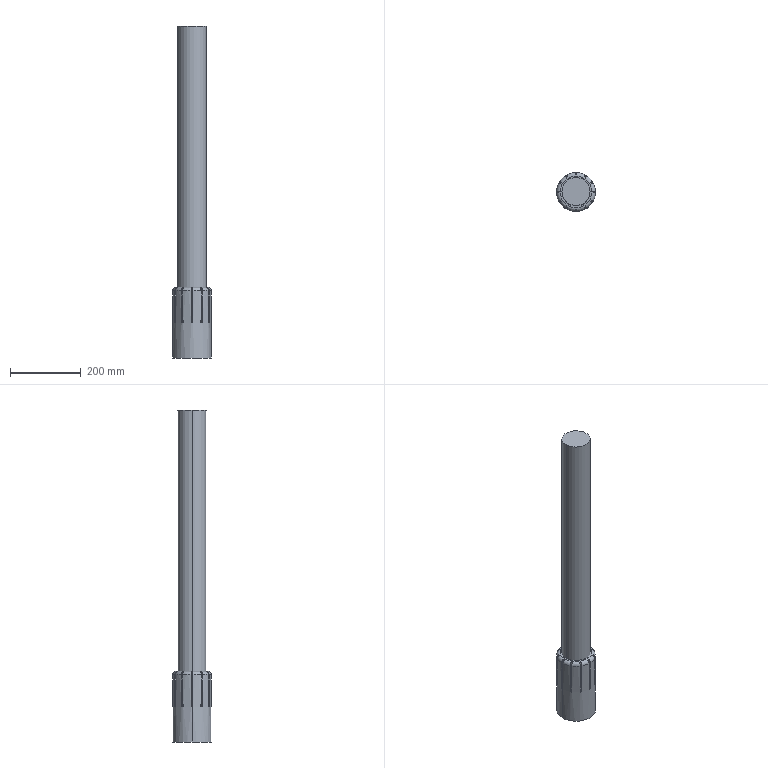Part | SolidWorks | features Cut 1, Extrusion 1, Fillet 1, ICE 1 | 1 solid | 58 faces | box 110 x 110 x 940 mm | volume 5584341 mm3 | plane 39 | cylinder 17 | torus 2 | commonest cylinder face diameters 100 x13 80 x2 110 x2